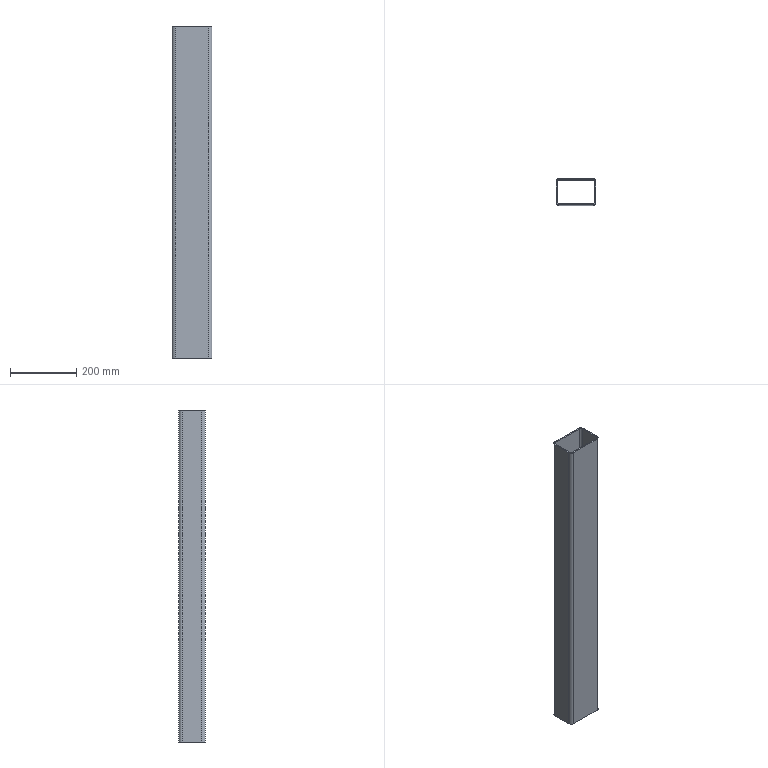Part | SolidWorks | features Extrusion 1, Fillet 1, Shell 1 | 1 solid | 18 faces | box 120 x 80 x 1002 mm | volume 1484024 mm3 | plane 10 | cylinder 8 | commonest cylinder face diameters 12 x4 20 x4
STEP:
#1=CARTESIAN_POINT('',(-50.,-40.,0.));
#2=VERTEX_POINT('',#1);
#3=CARTESIAN_POINT('',(50.,-40.,0.));
#4=VERTEX_POINT('',#3);
#5=CARTESIAN_POINT('',(60.,-40.,0.));
#6=DIRECTION('',(1.,0.,0.));
#7=VECTOR('',#6,1000.);
#8=LINE('',#5,#7);
#9=EDGE_CURVE('',#2,#4,#8,.T.);
#10=ORIENTED_EDGE('',*,*,#9,.F.);
#11=CARTESIAN_POINT('',(-60.,-30.,0.));
#12=VERTEX_POINT('',#11);
#13=CARTESIAN_POINT('',(-50.,-30.,0.));
#14=DIRECTION('',(0.,0.,-1.));
#15=DIRECTION('',(-1.,0.,0.));
#16=AXIS2_PLACEMENT_3D('',#13,#14,#15);
#17=CIRCLE('',#16,10.);
#18=EDGE_CURVE('',#2,#12,#17,.T.);
#19=ORIENTED_EDGE('',*,*,#18,.T.);
#20=CARTESIAN_POINT('',(-60.,30.,0.));
#21=VERTEX_POINT('',#20);
#22=CARTESIAN_POINT('',(-60.,40.,0.));
#23=DIRECTION('',(0.,-1.,0.));
#24=VECTOR('',#23,1000.);
#25=LINE('',#22,#24);
#26=EDGE_CURVE('',#21,#12,#25,.T.);
#27=ORIENTED_EDGE('',*,*,#26,.F.);
#28=CARTESIAN_POINT('',(-50.,40.,0.));
#29=VERTEX_POINT('',#28);
#30=CARTESIAN_POINT('',(-50.,30.,0.));
#31=DIRECTION('',(0.,0.,-1.));
#32=DIRECTION('',(-1.,0.,0.));
#33=AXIS2_PLACEMENT_3D('',#30,#31,#32);
#34=CIRCLE('',#33,10.);
#35=EDGE_CURVE('',#21,#29,#34,.T.);
#36=ORIENTED_EDGE('',*,*,#35,.T.);
#37=CARTESIAN_POINT('',(50.,40.,0.));
#38=VERTEX_POINT('',#37);
#39=CARTESIAN_POINT('',(60.,40.,0.));
#40=DIRECTION('',(-1.,0.,0.));
#41=VECTOR('',#40,1000.);
#42=LINE('',#39,#41);
#43=EDGE_CURVE('',#38,#29,#42,.T.);
#44=ORIENTED_EDGE('',*,*,#43,.F.);
#45=CARTESIAN_POINT('',(60.,30.,0.));
#46=VERTEX_POINT('',#45);
#47=CARTESIAN_POINT('',(50.,30.,0.));
#48=DIRECTION('',(0.,0.,-1.));
#49=DIRECTION('',(-1.,0.,0.));
#50=AXIS2_PLACEMENT_3D('',#47,#48,#49);
#51=CIRCLE('',#50,10.);
#52=EDGE_CURVE('',#38,#46,#51,.T.);
#53=ORIENTED_EDGE('',*,*,#52,.T.);
#54=CARTESIAN_POINT('',(60.,-30.,0.));
#55=VERTEX_POINT('',#54);
#56=CARTESIAN_POINT('',(60.,40.,0.));
#57=DIRECTION('',(0.,1.,0.));
#58=VECTOR('',#57,1000.);
#59=LINE('',#56,#58);
#60=EDGE_CURVE('',#55,#46,#59,.T.);
#61=ORIENTED_EDGE('',*,*,#60,.F.);
#62=CARTESIAN_POINT('',(50.,-30.,0.));
#63=DIRECTION('',(0.,0.,-1.));
#64=DIRECTION('',(-1.,0.,0.));
#65=AXIS2_PLACEMENT_3D('',#62,#63,#64);
#66=CIRCLE('',#65,10.);
#67=EDGE_CURVE('',#55,#4,#66,.T.);
#68=ORIENTED_EDGE('',*,*,#67,.T.);
#69=EDGE_LOOP('',(#10,#19,#27,#36,#44,#53,#61,#68));
#70=FACE_OUTER_BOUND('',#69,.T.);
#71=CARTESIAN_POINT('',(-50.,-36.,0.));
#72=VERTEX_POINT('',#71);
#73=CARTESIAN_POINT('',(-56.,-30.,0.));
#74=VERTEX_POINT('',#73);
#75=CARTESIAN_POINT('',(-50.,-30.,0.));
#76=DIRECTION('',(0.,0.,-1.));
#77=DIRECTION('',(-1.,0.,0.));
#78=AXIS2_PLACEMENT_3D('',#75,#76,#77);
#79=CIRCLE('',#78,6.);
#80=EDGE_CURVE('',#72,#74,#79,.T.);
#81=ORIENTED_EDGE('',*,*,#80,.F.);
#82=CARTESIAN_POINT('',(50.,-36.,0.));
#83=VERTEX_POINT('',#82);
#84=CARTESIAN_POINT('',(0.,-36.,0.));
#85=DIRECTION('',(1.,0.,0.));
#86=VECTOR('',#85,1000.);
#87=LINE('',#84,#86);
#88=EDGE_CURVE('',#72,#83,#87,.T.);
#89=ORIENTED_EDGE('',*,*,#88,.T.);
#90=CARTESIAN_POINT('',(56.,-30.,0.));
#91=VERTEX_POINT('',#90);
#92=CARTESIAN_POINT('',(50.,-30.,0.));
#93=DIRECTION('',(0.,0.,-1.));
#94=DIRECTION('',(-1.,0.,0.));
#95=AXIS2_PLACEMENT_3D('',#92,#93,#94);
#96=CIRCLE('',#95,6.);
#97=EDGE_CURVE('',#91,#83,#96,.T.);
#98=ORIENTED_EDGE('',*,*,#97,.F.);
#99=CARTESIAN_POINT('',(56.,30.,0.));
#100=VERTEX_POINT('',#99);
#101=CARTESIAN_POINT('',(56.,0.,0.));
#102=DIRECTION('',(0.,1.,0.));
#103=VECTOR('',#102,1000.);
#104=LINE('',#101,#103);
#105=EDGE_CURVE('',#91,#100,#104,.T.);
#106=ORIENTED_EDGE('',*,*,#105,.T.);
#107=CARTESIAN_POINT('',(50.,36.,0.));
#108=VERTEX_POINT('',#107);
#109=CARTESIAN_POINT('',(50.,30.,0.));
#110=DIRECTION('',(0.,0.,-1.));
#111=DIRECTION('',(-1.,0.,0.));
#112=AXIS2_PLACEMENT_3D('',#109,#110,#111);
#113=CIRCLE('',#112,6.);
#114=EDGE_CURVE('',#108,#100,#113,.T.);
#115=ORIENTED_EDGE('',*,*,#114,.F.);
#116=CARTESIAN_POINT('',(-50.,36.,0.));
#117=VERTEX_POINT('',#116);
#118=CARTESIAN_POINT('',(0.,36.,0.));
#119=DIRECTION('',(-1.,0.,0.));
#120=VECTOR('',#119,1000.);
#121=LINE('',#118,#120);
#122=EDGE_CURVE('',#108,#117,#121,.T.);
#123=ORIENTED_EDGE('',*,*,#122,.T.);
#124=CARTESIAN_POINT('',(-56.,30.,0.));
#125=VERTEX_POINT('',#124);
#126=CARTESIAN_POINT('',(-50.,30.,0.));
#127=DIRECTION('',(0.,0.,-1.));
#128=DIRECTION('',(-1.,0.,0.));
#129=AXIS2_PLACEMENT_3D('',#126,#127,#128);
#130=CIRCLE('',#129,6.);
#131=EDGE_CURVE('',#125,#117,#130,.T.);
#132=ORIENTED_EDGE('',*,*,#131,.F.);
#133=CARTESIAN_POINT('',(-56.,0.,0.));
#134=DIRECTION('',(0.,-1.,0.));
#135=VECTOR('',#134,1000.);
#136=LINE('',#133,#135);
#137=EDGE_CURVE('',#125,#74,#136,.T.);
#138=ORIENTED_EDGE('',*,*,#137,.T.);
#139=EDGE_LOOP('',(#81,#89,#98,#106,#115,#123,#132,#138));
#140=FACE_BOUND('',#139,.T.);
#141=CARTESIAN_POINT('',(0.,0.,0.));
#142=DIRECTION('',(0.,0.,-1.));
#143=DIRECTION('',(-1.,0.,0.));
#144=AXIS2_PLACEMENT_3D('',#141,#142,#143);
#145=PLANE('',#144);
#146=ADVANCED_FACE('',(#70,#140),#145,.T.);
#147=ORIENTED_EDGE('',*,*,#26,.T.);
#148=CARTESIAN_POINT('',(-60.,-30.,1002.));
#149=VERTEX_POINT('',#148);
#150=CARTESIAN_POINT('',(-60.,-30.,1002.));
#151=DIRECTION('',(0.,0.,1.));
#152=VECTOR('',#151,1000.);
#153=LINE('',#150,#152);
#154=EDGE_CURVE('',#12,#149,#153,.T.);
#155=ORIENTED_EDGE('',*,*,#154,.T.);
#156=CARTESIAN_POINT('',(-60.,30.,1002.));
#157=VERTEX_POINT('',#156);
#158=CARTESIAN_POINT('',(-60.,40.,1002.));
#159=DIRECTION('',(0.,-1.,0.));
#160=VECTOR('',#159,1000.);
#161=LINE('',#158,#160);
#162=EDGE_CURVE('',#157,#149,#161,.T.);
#163=ORIENTED_EDGE('',*,*,#162,.F.);
#164=CARTESIAN_POINT('',(-60.,30.,1002.));
#165=DIRECTION('',(0.,0.,-1.));
#166=VECTOR('',#165,1000.);
#167=LINE('',#164,#166);
#168=EDGE_CURVE('',#157,#21,#167,.T.);
#169=ORIENTED_EDGE('',*,*,#168,.T.);
#170=EDGE_LOOP('',(#147,#155,#163,#169));
#171=FACE_OUTER_BOUND('',#170,.T.);
#172=CARTESIAN_POINT('',(-60.,40.,1002.));
#173=DIRECTION('',(1.,0.,0.));
#174=DIRECTION('',(0.,1.,0.));
#175=AXIS2_PLACEMENT_3D('',#172,#173,#174);
#176=PLANE('',#175);
#177=ADVANCED_FACE('',(#171),#176,.F.);
#178=CARTESIAN_POINT('',(-50.,-40.,1002.));
#179=VERTEX_POINT('',#178);
#180=CARTESIAN_POINT('',(50.,-40.,1002.));
#181=VERTEX_POINT('',#180);
#182=CARTESIAN_POINT('',(60.,-40.,1002.));
#183=DIRECTION('',(1.,0.,0.));
#184=VECTOR('',#183,1000.);
#185=LINE('',#182,#184);
#186=EDGE_CURVE('',#179,#181,#185,.T.);
#187=ORIENTED_EDGE('',*,*,#186,.F.);
#188=CARTESIAN_POINT('',(-50.,-40.,1002.));
#189=DIRECTION('',(0.,0.,-1.));
#190=VECTOR('',#189,1000.);
#191=LINE('',#188,#190);
#192=EDGE_CURVE('',#179,#2,#191,.T.);
#193=ORIENTED_EDGE('',*,*,#192,.T.);
#194=ORIENTED_EDGE('',*,*,#9,.T.);
#195=CARTESIAN_POINT('',(50.,-40.,1002.));
#196=DIRECTION('',(0.,0.,1.));
#197=VECTOR('',#196,1000.);
#198=LINE('',#195,#197);
#199=EDGE_CURVE('',#4,#181,#198,.T.);
#200=ORIENTED_EDGE('',*,*,#199,.T.);
#201=EDGE_LOOP('',(#187,#193,#194,#200));
#202=FACE_OUTER_BOUND('',#201,.T.);
#203=CARTESIAN_POINT('',(60.,-40.,1002.));
#204=DIRECTION('',(0.,1.,0.));
#205=DIRECTION('',(-1.,0.,0.));
#206=AXIS2_PLACEMENT_3D('',#203,#204,#205);
#207=PLANE('',#206);
#208=ADVANCED_FACE('',(#202),#207,.F.);
#209=CARTESIAN_POINT('',(60.,-30.,1002.));
#210=VERTEX_POINT('',#209);
#211=CARTESIAN_POINT('',(60.,30.,1002.));
#212=VERTEX_POINT('',#211);
#213=CARTESIAN_POINT('',(60.,40.,1002.));
#214=DIRECTION('',(0.,1.,0.));
#215=VECTOR('',#214,1000.);
#216=LINE('',#213,#215);
#217=EDGE_CURVE('',#210,#212,#216,.T.);
#218=ORIENTED_EDGE('',*,*,#217,.F.);
#219=CARTESIAN_POINT('',(60.,-30.,1002.));
#220=DIRECTION('',(0.,0.,-1.));
#221=VECTOR('',#220,1000.);
#222=LINE('',#219,#221);
#223=EDGE_CURVE('',#210,#55,#222,.T.);
#224=ORIENTED_EDGE('',*,*,#223,.T.);
#225=ORIENTED_EDGE('',*,*,#60,.T.);
#226=CARTESIAN_POINT('',(60.,30.,1002.));
#227=DIRECTION('',(0.,0.,1.));
#228=VECTOR('',#227,1000.);
#229=LINE('',#226,#228);
#230=EDGE_CURVE('',#46,#212,#229,.T.);
#231=ORIENTED_EDGE('',*,*,#230,.T.);
#232=EDGE_LOOP('',(#218,#224,#225,#231));
#233=FACE_OUTER_BOUND('',#232,.T.);
#234=CARTESIAN_POINT('',(60.,40.,1002.));
#235=DIRECTION('',(-1.,0.,0.));
#236=DIRECTION('',(0.,-1.,0.));
#237=AXIS2_PLACEMENT_3D('',#234,#235,#236);
#238=PLANE('',#237);
#239=ADVANCED_FACE('',(#233),#238,.F.);
#240=CARTESIAN_POINT('',(50.,40.,1002.));
#241=VERTEX_POINT('',#240);
#242=CARTESIAN_POINT('',(-50.,40.,1002.));
#243=VERTEX_POINT('',#242);
#244=CARTESIAN_POINT('',(60.,40.,1002.));
#245=DIRECTION('',(-1.,0.,0.));
#246=VECTOR('',#245,1000.);
#247=LINE('',#244,#246);
#248=EDGE_CURVE('',#241,#243,#247,.T.);
#249=ORIENTED_EDGE('',*,*,#248,.F.);
#250=CARTESIAN_POINT('',(50.,40.,1002.));
#251=DIRECTION('',(0.,0.,-1.));
#252=VECTOR('',#251,1000.);
#253=LINE('',#250,#252);
#254=EDGE_CURVE('',#241,#38,#253,.T.);
#255=ORIENTED_EDGE('',*,*,#254,.T.);
#256=ORIENTED_EDGE('',*,*,#43,.T.);
#257=CARTESIAN_POINT('',(-50.,40.,1002.));
#258=DIRECTION('',(0.,0.,1.));
#259=VECTOR('',#258,1000.);
#260=LINE('',#257,#259);
#261=EDGE_CURVE('',#29,#243,#260,.T.);
#262=ORIENTED_EDGE('',*,*,#261,.T.);
#263=EDGE_LOOP('',(#249,#255,#256,#262));
#264=FACE_OUTER_BOUND('',#263,.T.);
#265=CARTESIAN_POINT('',(60.,40.,1002.));
#266=DIRECTION('',(0.,-1.,0.));
#267=DIRECTION('',(1.,0.,0.));
#268=AXIS2_PLACEMENT_3D('',#265,#266,#267);
#269=PLANE('',#268);
#270=ADVANCED_FACE('',(#264),#269,.F.);
#271=CARTESIAN_POINT('',(-56.,30.,1002.));
#272=VERTEX_POINT('',#271);
#273=CARTESIAN_POINT('',(-56.,-30.,1002.));
#274=VERTEX_POINT('',#273);
#275=CARTESIAN_POINT('',(-56.,0.,1002.));
#276=DIRECTION('',(0.,-1.,0.));
#277=VECTOR('',#276,1000.);
#278=LINE('',#275,#277);
#279=EDGE_CURVE('',#272,#274,#278,.T.);
#280=ORIENTED_EDGE('',*,*,#279,.F.);
#281=CARTESIAN_POINT('',(-50.,36.,1002.));
#282=VERTEX_POINT('',#281);
#283=CARTESIAN_POINT('',(-50.,30.,1002.));
#284=DIRECTION('',(0.,0.,1.));
#285=DIRECTION('',(-1.,0.,0.));
#286=AXIS2_PLACEMENT_3D('',#283,#284,#285);
#287=CIRCLE('',#286,6.);
#288=EDGE_CURVE('',#282,#272,#287,.T.);
#289=ORIENTED_EDGE('',*,*,#288,.F.);
#290=CARTESIAN_POINT('',(50.,36.,1002.));
#291=VERTEX_POINT('',#290);
#292=CARTESIAN_POINT('',(0.,36.,1002.));
#293=DIRECTION('',(-1.,0.,0.));
#294=VECTOR('',#293,1000.);
#295=LINE('',#292,#294);
#296=EDGE_CURVE('',#291,#282,#295,.T.);
#297=ORIENTED_EDGE('',*,*,#296,.F.);
#298=CARTESIAN_POINT('',(56.,30.,1002.));
#299=VERTEX_POINT('',#298);
#300=CARTESIAN_POINT('',(50.,30.,1002.));
#301=DIRECTION('',(0.,0.,1.));
#302=DIRECTION('',(-1.,0.,0.));
#303=AXIS2_PLACEMENT_3D('',#300,#301,#302);
#304=CIRCLE('',#303,6.);
#305=EDGE_CURVE('',#299,#291,#304,.T.);
#306=ORIENTED_EDGE('',*,*,#305,.F.);
#307=CARTESIAN_POINT('',(56.,-30.,1002.));
#308=VERTEX_POINT('',#307);
#309=CARTESIAN_POINT('',(56.,0.,1002.));
#310=DIRECTION('',(0.,1.,0.));
#311=VECTOR('',#310,1000.);
#312=LINE('',#309,#311);
#313=EDGE_CURVE('',#308,#299,#312,.T.);
#314=ORIENTED_EDGE('',*,*,#313,.F.);
#315=CARTESIAN_POINT('',(50.,-36.,1002.));
#316=VERTEX_POINT('',#315);
#317=CARTESIAN_POINT('',(50.,-30.,1002.));
#318=DIRECTION('',(0.,0.,1.));
#319=DIRECTION('',(-1.,0.,0.));
#320=AXIS2_PLACEMENT_3D('',#317,#318,#319);
#321=CIRCLE('',#320,6.);
#322=EDGE_CURVE('',#316,#308,#321,.T.);
#323=ORIENTED_EDGE('',*,*,#322,.F.);
#324=CARTESIAN_POINT('',(-50.,-36.,1002.));
#325=VERTEX_POINT('',#324);
#326=CARTESIAN_POINT('',(0.,-36.,1002.));
#327=DIRECTION('',(1.,0.,0.));
#328=VECTOR('',#327,1000.);
#329=LINE('',#326,#328);
#330=EDGE_CURVE('',#325,#316,#329,.T.);
#331=ORIENTED_EDGE('',*,*,#330,.F.);
#332=CARTESIAN_POINT('',(-50.,-30.,1002.));
#333=DIRECTION('',(0.,0.,1.));
#334=DIRECTION('',(-1.,0.,0.));
#335=AXIS2_PLACEMENT_3D('',#332,#333,#334);
#336=CIRCLE('',#335,6.);
#337=EDGE_CURVE('',#274,#325,#336,.T.);
#338=ORIENTED_EDGE('',*,*,#337,.F.);
#339=EDGE_LOOP('',(#280,#289,#297,#306,#314,#323,#331,#338));
#340=FACE_BOUND('',#339,.T.);
#341=ORIENTED_EDGE('',*,*,#162,.T.);
#342=CARTESIAN_POINT('',(-50.,-30.,1002.));
#343=DIRECTION('',(0.,0.,1.));
#344=DIRECTION('',(-1.,0.,0.));
#345=AXIS2_PLACEMENT_3D('',#342,#343,#344);
#346=CIRCLE('',#345,10.);
#347=EDGE_CURVE('',#149,#179,#346,.T.);
#348=ORIENTED_EDGE('',*,*,#347,.T.);
#349=ORIENTED_EDGE('',*,*,#186,.T.);
#350=CARTESIAN_POINT('',(50.,-30.,1002.));
#351=DIRECTION('',(0.,0.,1.));
#352=DIRECTION('',(-1.,0.,0.));
#353=AXIS2_PLACEMENT_3D('',#350,#351,#352);
#354=CIRCLE('',#353,10.);
#355=EDGE_CURVE('',#181,#210,#354,.T.);
#356=ORIENTED_EDGE('',*,*,#355,.T.);
#357=ORIENTED_EDGE('',*,*,#217,.T.);
#358=CARTESIAN_POINT('',(50.,30.,1002.));
#359=DIRECTION('',(0.,0.,1.));
#360=DIRECTION('',(-1.,0.,0.));
#361=AXIS2_PLACEMENT_3D('',#358,#359,#360);
#362=CIRCLE('',#361,10.);
#363=EDGE_CURVE('',#212,#241,#362,.T.);
#364=ORIENTED_EDGE('',*,*,#363,.T.);
#365=ORIENTED_EDGE('',*,*,#248,.T.);
#366=CARTESIAN_POINT('',(-50.,30.,1002.));
#367=DIRECTION('',(0.,0.,1.));
#368=DIRECTION('',(-1.,0.,0.));
#369=AXIS2_PLACEMENT_3D('',#366,#367,#368);
#370=CIRCLE('',#369,10.);
#371=EDGE_CURVE('',#243,#157,#370,.T.);
#372=ORIENTED_EDGE('',*,*,#371,.T.);
#373=EDGE_LOOP('',(#341,#348,#349,#356,#357,#364,#365,#372));
#374=FACE_OUTER_BOUND('',#373,.T.);
#375=CARTESIAN_POINT('',(0.,0.,1002.));
#376=DIRECTION('',(0.,0.,-1.));
#377=DIRECTION('',(-1.,0.,0.));
#378=AXIS2_PLACEMENT_3D('',#375,#376,#377);
#379=PLANE('',#378);
#380=ADVANCED_FACE('',(#340,#374),#379,.F.);
#381=ORIENTED_EDGE('',*,*,#347,.F.);
#382=ORIENTED_EDGE('',*,*,#154,.F.);
#383=ORIENTED_EDGE('',*,*,#18,.F.);
#384=ORIENTED_EDGE('',*,*,#192,.F.);
#385=EDGE_LOOP('',(#381,#382,#383,#384));
#386=FACE_OUTER_BOUND('',#385,.T.);
#387=CARTESIAN_POINT('',(-50.,-30.,1002.));
#388=DIRECTION('',(0.,0.,-1.));
#389=DIRECTION('',(-1.,0.,0.));
#390=AXIS2_PLACEMENT_3D('',#387,#388,#389);
#391=CYLINDRICAL_SURFACE('',#390,10.);
#392=ADVANCED_FACE('',(#386),#391,.T.);
#393=ORIENTED_EDGE('',*,*,#355,.F.);
#394=ORIENTED_EDGE('',*,*,#199,.F.);
#395=ORIENTED_EDGE('',*,*,#67,.F.);
#396=ORIENTED_EDGE('',*,*,#223,.F.);
#397=EDGE_LOOP('',(#393,#394,#395,#396));
#398=FACE_OUTER_BOUND('',#397,.T.);
#399=CARTESIAN_POINT('',(50.,-30.,1002.));
#400=DIRECTION('',(0.,0.,-1.));
#401=DIRECTION('',(-1.,0.,0.));
#402=AXIS2_PLACEMENT_3D('',#399,#400,#401);
#403=CYLINDRICAL_SURFACE('',#402,10.);
#404=ADVANCED_FACE('',(#398),#403,.T.);
#405=ORIENTED_EDGE('',*,*,#363,.F.);
#406=ORIENTED_EDGE('',*,*,#230,.F.);
#407=ORIENTED_EDGE('',*,*,#52,.F.);
#408=ORIENTED_EDGE('',*,*,#254,.F.);
#409=EDGE_LOOP('',(#405,#406,#407,#408));
#410=FACE_OUTER_BOUND('',#409,.T.);
#411=CARTESIAN_POINT('',(50.,30.,1002.));
#412=DIRECTION('',(0.,0.,-1.));
#413=DIRECTION('',(-1.,0.,0.));
#414=AXIS2_PLACEMENT_3D('',#411,#412,#413);
#415=CYLINDRICAL_SURFACE('',#414,10.);
#416=ADVANCED_FACE('',(#410),#415,.T.);
#417=ORIENTED_EDGE('',*,*,#371,.F.);
#418=ORIENTED_EDGE('',*,*,#261,.F.);
#419=ORIENTED_EDGE('',*,*,#35,.F.);
#420=ORIENTED_EDGE('',*,*,#168,.F.);
#421=EDGE_LOOP('',(#417,#418,#419,#420));
#422=FACE_OUTER_BOUND('',#421,.T.);
#423=CARTESIAN_POINT('',(-50.,30.,1002.));
#424=DIRECTION('',(0.,0.,-1.));
#425=DIRECTION('',(-1.,0.,0.));
#426=AXIS2_PLACEMENT_3D('',#423,#424,#425);
#427=CYLINDRICAL_SURFACE('',#426,10.);
#428=ADVANCED_FACE('',(#422),#427,.T.);
#429=ORIENTED_EDGE('',*,*,#137,.F.);
#430=CARTESIAN_POINT('',(-56.,30.,1002.));
#431=DIRECTION('',(0.,0.,-1.));
#432=VECTOR('',#431,1000.);
#433=LINE('',#430,#432);
#434=EDGE_CURVE('',#272,#125,#433,.T.);
#435=ORIENTED_EDGE('',*,*,#434,.F.);
#436=ORIENTED_EDGE('',*,*,#279,.T.);
#437=CARTESIAN_POINT('',(-56.,-30.,1002.));
#438=DIRECTION('',(0.,0.,1.));
#439=VECTOR('',#438,1000.);
#440=LINE('',#437,#439);
#441=EDGE_CURVE('',#74,#274,#440,.T.);
#442=ORIENTED_EDGE('',*,*,#441,.F.);
#443=EDGE_LOOP('',(#429,#435,#436,#442));
#444=FACE_OUTER_BOUND('',#443,.T.);
#445=CARTESIAN_POINT('',(-56.,40.,1002.));
#446=DIRECTION('',(1.,0.,0.));
#447=DIRECTION('',(0.,1.,0.));
#448=AXIS2_PLACEMENT_3D('',#445,#446,#447);
#449=PLANE('',#448);
#450=ADVANCED_FACE('',(#444),#449,.T.);
#451=ORIENTED_EDGE('',*,*,#330,.T.);
#452=CARTESIAN_POINT('',(50.,-36.,1002.));
#453=DIRECTION('',(0.,0.,1.));
#454=VECTOR('',#453,1000.);
#455=LINE('',#452,#454);
#456=EDGE_CURVE('',#83,#316,#455,.T.);
#457=ORIENTED_EDGE('',*,*,#456,.F.);
#458=ORIENTED_EDGE('',*,*,#88,.F.);
#459=CARTESIAN_POINT('',(-50.,-36.,1002.));
#460=DIRECTION('',(0.,0.,-1.));
#461=VECTOR('',#460,1000.);
#462=LINE('',#459,#461);
#463=EDGE_CURVE('',#325,#72,#462,.T.);
#464=ORIENTED_EDGE('',*,*,#463,.F.);
#465=EDGE_LOOP('',(#451,#457,#458,#464));
#466=FACE_OUTER_BOUND('',#465,.T.);
#467=CARTESIAN_POINT('',(60.,-36.,1002.));
#468=DIRECTION('',(0.,1.,0.));
#469=DIRECTION('',(-1.,0.,0.));
#470=AXIS2_PLACEMENT_3D('',#467,#468,#469);
#471=PLANE('',#470);
#472=ADVANCED_FACE('',(#466),#471,.T.);
#473=ORIENTED_EDGE('',*,*,#313,.T.);
#474=CARTESIAN_POINT('',(56.,30.,1002.));
#475=DIRECTION('',(0.,0.,1.));
#476=VECTOR('',#475,1000.);
#477=LINE('',#474,#476);
#478=EDGE_CURVE('',#100,#299,#477,.T.);
#479=ORIENTED_EDGE('',*,*,#478,.F.);
#480=ORIENTED_EDGE('',*,*,#105,.F.);
#481=CARTESIAN_POINT('',(56.,-30.,1002.));
#482=DIRECTION('',(0.,0.,-1.));
#483=VECTOR('',#482,1000.);
#484=LINE('',#481,#483);
#485=EDGE_CURVE('',#308,#91,#484,.T.);
#486=ORIENTED_EDGE('',*,*,#485,.F.);
#487=EDGE_LOOP('',(#473,#479,#480,#486));
#488=FACE_OUTER_BOUND('',#487,.T.);
#489=CARTESIAN_POINT('',(56.,40.,1002.));
#490=DIRECTION('',(-1.,0.,0.));
#491=DIRECTION('',(0.,-1.,0.));
#492=AXIS2_PLACEMENT_3D('',#489,#490,#491);
#493=PLANE('',#492);
#494=ADVANCED_FACE('',(#488),#493,.T.);
#495=ORIENTED_EDGE('',*,*,#296,.T.);
#496=CARTESIAN_POINT('',(-50.,36.,1002.));
#497=DIRECTION('',(0.,0.,1.));
#498=VECTOR('',#497,1000.);
#499=LINE('',#496,#498);
#500=EDGE_CURVE('',#117,#282,#499,.T.);
#501=ORIENTED_EDGE('',*,*,#500,.F.);
#502=ORIENTED_EDGE('',*,*,#122,.F.);
#503=CARTESIAN_POINT('',(50.,36.,1002.));
#504=DIRECTION('',(0.,0.,-1.));
#505=VECTOR('',#504,1000.);
#506=LINE('',#503,#505);
#507=EDGE_CURVE('',#291,#108,#506,.T.);
#508=ORIENTED_EDGE('',*,*,#507,.F.);
#509=EDGE_LOOP('',(#495,#501,#502,#508));
#510=FACE_OUTER_BOUND('',#509,.T.);
#511=CARTESIAN_POINT('',(60.,36.,1002.));
#512=DIRECTION('',(0.,-1.,0.));
#513=DIRECTION('',(1.,0.,0.));
#514=AXIS2_PLACEMENT_3D('',#511,#512,#513);
#515=PLANE('',#514);
#516=ADVANCED_FACE('',(#510),#515,.T.);
#517=ORIENTED_EDGE('',*,*,#337,.T.);
#518=ORIENTED_EDGE('',*,*,#463,.T.);
#519=ORIENTED_EDGE('',*,*,#80,.T.);
#520=ORIENTED_EDGE('',*,*,#441,.T.);
#521=EDGE_LOOP('',(#517,#518,#519,#520));
#522=FACE_OUTER_BOUND('',#521,.T.);
#523=CARTESIAN_POINT('',(-50.,-30.,1002.));
#524=DIRECTION('',(0.,0.,-1.));
#525=DIRECTION('',(-1.,0.,0.));
#526=AXIS2_PLACEMENT_3D('',#523,#524,#525);
#527=CYLINDRICAL_SURFACE('',#526,6.);
#528=ADVANCED_FACE('',(#522),#527,.F.);
#529=ORIENTED_EDGE('',*,*,#322,.T.);
#530=ORIENTED_EDGE('',*,*,#485,.T.);
#531=ORIENTED_EDGE('',*,*,#97,.T.);
#532=ORIENTED_EDGE('',*,*,#456,.T.);
#533=EDGE_LOOP('',(#529,#530,#531,#532));
#534=FACE_OUTER_BOUND('',#533,.T.);
#535=CARTESIAN_POINT('',(50.,-30.,1002.));
#536=DIRECTION('',(0.,0.,-1.));
#537=DIRECTION('',(-1.,0.,0.));
#538=AXIS2_PLACEMENT_3D('',#535,#536,#537);
#539=CYLINDRICAL_SURFACE('',#538,6.);
#540=ADVANCED_FACE('',(#534),#539,.F.);
#541=ORIENTED_EDGE('',*,*,#305,.T.);
#542=ORIENTED_EDGE('',*,*,#507,.T.);
#543=ORIENTED_EDGE('',*,*,#114,.T.);
#544=ORIENTED_EDGE('',*,*,#478,.T.);
#545=EDGE_LOOP('',(#541,#542,#543,#544));
#546=FACE_OUTER_BOUND('',#545,.T.);
#547=CARTESIAN_POINT('',(50.,30.,1002.));
#548=DIRECTION('',(0.,0.,-1.));
#549=DIRECTION('',(-1.,0.,0.));
#550=AXIS2_PLACEMENT_3D('',#547,#548,#549);
#551=CYLINDRICAL_SURFACE('',#550,6.);
#552=ADVANCED_FACE('',(#546),#551,.F.);
#553=ORIENTED_EDGE('',*,*,#288,.T.);
#554=ORIENTED_EDGE('',*,*,#434,.T.);
#555=ORIENTED_EDGE('',*,*,#131,.T.);
#556=ORIENTED_EDGE('',*,*,#500,.T.);
#557=EDGE_LOOP('',(#553,#554,#555,#556));
#558=FACE_OUTER_BOUND('',#557,.T.);
#559=CARTESIAN_POINT('',(-50.,30.,1002.));
#560=DIRECTION('',(0.,0.,-1.));
#561=DIRECTION('',(-1.,0.,0.));
#562=AXIS2_PLACEMENT_3D('',#559,#560,#561);
#563=CYLINDRICAL_SURFACE('',#562,6.);
#564=ADVANCED_FACE('',(#558),#563,.F.);
#565=CLOSED_SHELL('',(#146,#177,#208,#239,#270,#380,#392,#404,#416,#428,#450,#472,#494,#516,#528,#540,#552,#564));
#566=MANIFOLD_SOLID_BREP('',#565);
#567=CARTESIAN_POINT('',(0.,0.,0.));
#568=DIRECTION('',(0.,0.,1.));
#569=DIRECTION('',(1.,0.,0.));
#570=AXIS2_PLACEMENT_3D('',#567,#568,#569);
#571=(LENGTH_UNIT()NAMED_UNIT(*)SI_UNIT(.MILLI.,.METRE.));
#572=UNCERTAINTY_MEASURE_WITH_UNIT(LENGTH_MEASURE(0.00001),#571,'','');
#573=(NAMED_UNIT(*)PLANE_ANGLE_UNIT()SI_UNIT($,.RADIAN.));
#574=(NAMED_UNIT(*)SI_UNIT($,.STERADIAN.)SOLID_ANGLE_UNIT());
#575=(GEOMETRIC_REPRESENTATION_CONTEXT(3)GLOBAL_UNCERTAINTY_ASSIGNED_CONTEXT((#572))GLOBAL_UNIT_ASSIGNED_CONTEXT((#571,#573,#574))REPRESENTATION_CONTEXT('',''));
#576=ADVANCED_BREP_SHAPE_REPRESENTATION('',(#566,#570),#575);